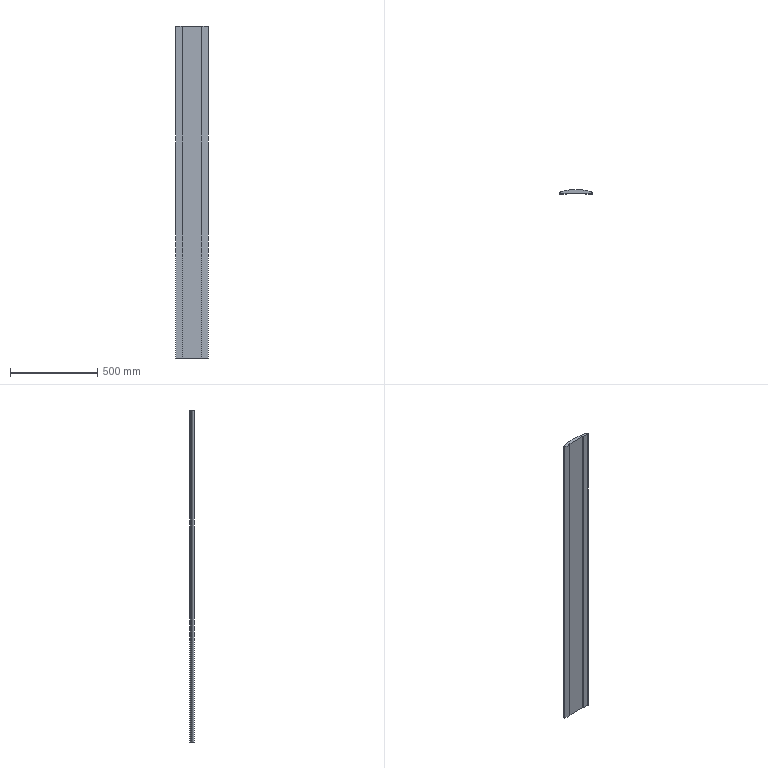Part | SolidWorks | features BaseBody 1 | 1 solid | 31 faces | box 188.037 x 25 x 1900 mm | volume 6268934 mm3 | cylinder 24 | plane 7 | commonest cylinder face diameters 0.2 x8 0.6 x6 661 x5 28 x3 0.4 x2
STEP:
#1=CARTESIAN_POINT('',(-94.018,0.7177,950.));
#2=VERTEX_POINT('',#1);
#3=CARTESIAN_POINT('',(-94.012,0.2909,950.));
#4=VERTEX_POINT('',#3);
#5=CARTESIAN_POINT('',(-80.018,0.7177,950.));
#6=DIRECTION('',(0.,0.,1.));
#7=DIRECTION('',(-1.,0.,0.));
#8=AXIS2_PLACEMENT_3D('',#5,#6,#7);
#9=CIRCLE('',#8,14.);
#10=EDGE_CURVE('',#2,#4,#9,.T.);
#11=ORIENTED_EDGE('',*,*,#10,.F.);
#12=CARTESIAN_POINT('',(-94.018,0.7177,-950.));
#13=VERTEX_POINT('',#12);
#14=CARTESIAN_POINT('',(-94.018,0.7177,950.));
#15=DIRECTION('',(0.,0.,-1.));
#16=VECTOR('',#15,1000.);
#17=LINE('',#14,#16);
#18=EDGE_CURVE('',#2,#13,#17,.T.);
#19=ORIENTED_EDGE('',*,*,#18,.T.);
#20=CARTESIAN_POINT('',(-94.012,0.2909,-950.));
#21=VERTEX_POINT('',#20);
#22=CARTESIAN_POINT('',(-80.018,0.7177,-950.));
#23=DIRECTION('',(0.,0.,1.));
#24=DIRECTION('',(-1.,0.,0.));
#25=AXIS2_PLACEMENT_3D('',#22,#23,#24);
#26=CIRCLE('',#25,14.);
#27=EDGE_CURVE('',#13,#21,#26,.T.);
#28=ORIENTED_EDGE('',*,*,#27,.T.);
#29=CARTESIAN_POINT('',(-94.012,0.2909,950.));
#30=DIRECTION('',(0.,0.,-1.));
#31=VECTOR('',#30,1000.);
#32=LINE('',#29,#31);
#33=EDGE_CURVE('',#4,#21,#32,.T.);
#34=ORIENTED_EDGE('',*,*,#33,.F.);
#35=EDGE_LOOP('',(#11,#19,#28,#34));
#36=FACE_OUTER_BOUND('',#35,.T.);
#37=CARTESIAN_POINT('',(-80.018,0.7177,950.));
#38=DIRECTION('',(0.,0.,-1.));
#39=DIRECTION('',(-1.,0.,0.));
#40=AXIS2_PLACEMENT_3D('',#37,#38,#39);
#41=CYLINDRICAL_SURFACE('',#40,14.);
#42=ADVANCED_FACE('',(#36),#41,.T.);
#43=CARTESIAN_POINT('',(-58.619,19.76,950.));
#44=VERTEX_POINT('',#43);
#45=CARTESIAN_POINT('',(58.619,19.76,950.));
#46=VERTEX_POINT('',#45);
#47=CARTESIAN_POINT('',(0.,-305.5,950.));
#48=DIRECTION('',(0.,0.,-1.));
#49=DIRECTION('',(-1.,0.,0.));
#50=AXIS2_PLACEMENT_3D('',#47,#48,#49);
#51=CIRCLE('',#50,330.5);
#52=EDGE_CURVE('',#44,#46,#51,.T.);
#53=ORIENTED_EDGE('',*,*,#52,.T.);
#54=CARTESIAN_POINT('',(58.619,19.76,-950.));
#55=VERTEX_POINT('',#54);
#56=CARTESIAN_POINT('',(58.619,19.76,950.));
#57=DIRECTION('',(0.,0.,-1.));
#58=VECTOR('',#57,1000.);
#59=LINE('',#56,#58);
#60=EDGE_CURVE('',#46,#55,#59,.T.);
#61=ORIENTED_EDGE('',*,*,#60,.T.);
#62=CARTESIAN_POINT('',(-58.619,19.76,-950.));
#63=VERTEX_POINT('',#62);
#64=CARTESIAN_POINT('',(0.,-305.5,-950.));
#65=DIRECTION('',(0.,0.,1.));
#66=DIRECTION('',(-1.,0.,0.));
#67=AXIS2_PLACEMENT_3D('',#64,#65,#66);
#68=CIRCLE('',#67,330.5);
#69=EDGE_CURVE('',#55,#63,#68,.T.);
#70=ORIENTED_EDGE('',*,*,#69,.T.);
#71=CARTESIAN_POINT('',(-58.619,19.76,950.));
#72=DIRECTION('',(0.,0.,1.));
#73=VECTOR('',#72,1000.);
#74=LINE('',#71,#73);
#75=EDGE_CURVE('',#63,#44,#74,.T.);
#76=ORIENTED_EDGE('',*,*,#75,.T.);
#77=EDGE_LOOP('',(#53,#61,#70,#76));
#78=FACE_OUTER_BOUND('',#77,.T.);
#79=CARTESIAN_POINT('',(0.,-305.5,950.));
#80=DIRECTION('',(0.,0.,-1.));
#81=DIRECTION('',(-1.,0.,0.));
#82=AXIS2_PLACEMENT_3D('',#79,#80,#81);
#83=CYLINDRICAL_SURFACE('',#82,330.5);
#84=ADVANCED_FACE('',(#78),#83,.T.);
#85=CARTESIAN_POINT('',(58.701,19.669,950.));
#86=VERTEX_POINT('',#85);
#87=CARTESIAN_POINT('',(58.601,19.662,950.));
#88=DIRECTION('',(0.,0.,-1.));
#89=DIRECTION('',(-1.,0.,0.));
#90=AXIS2_PLACEMENT_3D('',#87,#88,#89);
#91=CIRCLE('',#90,0.1);
#92=EDGE_CURVE('',#46,#86,#91,.T.);
#93=ORIENTED_EDGE('',*,*,#92,.T.);
#94=CARTESIAN_POINT('',(58.701,19.669,-950.));
#95=VERTEX_POINT('',#94);
#96=CARTESIAN_POINT('',(58.701,19.669,950.));
#97=DIRECTION('',(0.,0.,-1.));
#98=VECTOR('',#97,1000.);
#99=LINE('',#96,#98);
#100=EDGE_CURVE('',#86,#95,#99,.T.);
#101=ORIENTED_EDGE('',*,*,#100,.T.);
#102=CARTESIAN_POINT('',(58.601,19.662,-950.));
#103=DIRECTION('',(0.,0.,1.));
#104=DIRECTION('',(-1.,0.,0.));
#105=AXIS2_PLACEMENT_3D('',#102,#103,#104);
#106=CIRCLE('',#105,0.1);
#107=EDGE_CURVE('',#95,#55,#106,.T.);
#108=ORIENTED_EDGE('',*,*,#107,.T.);
#109=ORIENTED_EDGE('',*,*,#60,.F.);
#110=EDGE_LOOP('',(#93,#101,#108,#109));
#111=FACE_OUTER_BOUND('',#110,.T.);
#112=CARTESIAN_POINT('',(58.601,19.662,950.));
#113=DIRECTION('',(0.,0.,-1.));
#114=DIRECTION('',(-1.,0.,0.));
#115=AXIS2_PLACEMENT_3D('',#112,#113,#114);
#116=CYLINDRICAL_SURFACE('',#115,0.1);
#117=ADVANCED_FACE('',(#111),#116,.T.);
#118=CARTESIAN_POINT('',(-60.381,19.438,950.));
#119=VERTEX_POINT('',#118);
#120=CARTESIAN_POINT('',(-60.272,19.381,950.));
#121=VERTEX_POINT('',#120);
#122=CARTESIAN_POINT('',(-60.363,19.339,950.));
#123=DIRECTION('',(0.,0.,-1.));
#124=DIRECTION('',(-1.,0.,0.));
#125=AXIS2_PLACEMENT_3D('',#122,#123,#124);
#126=CIRCLE('',#125,0.1);
#127=EDGE_CURVE('',#119,#121,#126,.T.);
#128=ORIENTED_EDGE('',*,*,#127,.F.);
#129=CARTESIAN_POINT('',(-83.558,14.263,950.));
#130=VERTEX_POINT('',#129);
#131=CARTESIAN_POINT('',(0.,-305.5,950.));
#132=DIRECTION('',(0.,0.,1.));
#133=DIRECTION('',(-1.,0.,0.));
#134=AXIS2_PLACEMENT_3D('',#131,#132,#133);
#135=CIRCLE('',#134,330.5);
#136=EDGE_CURVE('',#119,#130,#135,.T.);
#137=ORIENTED_EDGE('',*,*,#136,.T.);
#138=CARTESIAN_POINT('',(-80.018,0.7177,950.));
#139=DIRECTION('',(0.,0.,1.));
#140=DIRECTION('',(-1.,0.,0.));
#141=AXIS2_PLACEMENT_3D('',#138,#139,#140);
#142=CIRCLE('',#141,14.);
#143=EDGE_CURVE('',#130,#2,#142,.T.);
#144=ORIENTED_EDGE('',*,*,#143,.T.);
#145=ORIENTED_EDGE('',*,*,#10,.T.);
#146=CARTESIAN_POINT('',(-93.712,0.,950.));
#147=VERTEX_POINT('',#146);
#148=CARTESIAN_POINT('',(-93.712,0.3,950.));
#149=DIRECTION('',(0.,0.,-1.));
#150=DIRECTION('',(-1.,0.,0.));
#151=AXIS2_PLACEMENT_3D('',#148,#149,#150);
#152=CIRCLE('',#151,0.3);
#153=EDGE_CURVE('',#147,#4,#152,.T.);
#154=ORIENTED_EDGE('',*,*,#153,.F.);
#155=CARTESIAN_POINT('',(-56.7,0.,950.));
#156=VERTEX_POINT('',#155);
#157=CARTESIAN_POINT('',(-80.018,0.,950.));
#158=DIRECTION('',(1.,0.,0.));
#159=VECTOR('',#158,1000.);
#160=LINE('',#157,#159);
#161=EDGE_CURVE('',#147,#156,#160,.T.);
#162=ORIENTED_EDGE('',*,*,#161,.T.);
#163=CARTESIAN_POINT('',(-56.5,0.2,950.));
#164=VERTEX_POINT('',#163);
#165=CARTESIAN_POINT('',(-56.7,0.2,950.));
#166=DIRECTION('',(0.,0.,-1.));
#167=DIRECTION('',(-1.,0.,0.));
#168=AXIS2_PLACEMENT_3D('',#165,#166,#167);
#169=CIRCLE('',#168,0.2);
#170=EDGE_CURVE('',#164,#156,#169,.T.);
#171=ORIENTED_EDGE('',*,*,#170,.F.);
#172=CARTESIAN_POINT('',(-56.5,4.5,950.));
#173=VERTEX_POINT('',#172);
#174=CARTESIAN_POINT('',(-56.5,0.7177,950.));
#175=DIRECTION('',(0.,1.,0.));
#176=VECTOR('',#175,1000.);
#177=LINE('',#174,#176);
#178=EDGE_CURVE('',#164,#173,#177,.T.);
#179=ORIENTED_EDGE('',*,*,#178,.T.);
#180=CARTESIAN_POINT('',(56.5,4.5,950.));
#181=VERTEX_POINT('',#180);
#182=CARTESIAN_POINT('',(-80.018,4.5,950.));
#183=DIRECTION('',(1.,0.,0.));
#184=VECTOR('',#183,1000.);
#185=LINE('',#182,#184);
#186=EDGE_CURVE('',#173,#181,#185,.T.);
#187=ORIENTED_EDGE('',*,*,#186,.T.);
#188=CARTESIAN_POINT('',(56.5,0.2,950.));
#189=VERTEX_POINT('',#188);
#190=CARTESIAN_POINT('',(56.5,0.7177,950.));
#191=DIRECTION('',(0.,-1.,0.));
#192=VECTOR('',#191,1000.);
#193=LINE('',#190,#192);
#194=EDGE_CURVE('',#181,#189,#193,.T.);
#195=ORIENTED_EDGE('',*,*,#194,.T.);
#196=CARTESIAN_POINT('',(56.7,0.,950.));
#197=VERTEX_POINT('',#196);
#198=CARTESIAN_POINT('',(56.7,0.2,950.));
#199=DIRECTION('',(0.,0.,-1.));
#200=DIRECTION('',(-1.,0.,0.));
#201=AXIS2_PLACEMENT_3D('',#198,#199,#200);
#202=CIRCLE('',#201,0.2);
#203=EDGE_CURVE('',#197,#189,#202,.T.);
#204=ORIENTED_EDGE('',*,*,#203,.F.);
#205=CARTESIAN_POINT('',(93.712,0.,950.));
#206=VERTEX_POINT('',#205);
#207=CARTESIAN_POINT('',(-80.018,0.,950.));
#208=DIRECTION('',(1.,0.,0.));
#209=VECTOR('',#208,1000.);
#210=LINE('',#207,#209);
#211=EDGE_CURVE('',#197,#206,#210,.T.);
#212=ORIENTED_EDGE('',*,*,#211,.T.);
#213=CARTESIAN_POINT('',(94.012,0.2909,950.));
#214=VERTEX_POINT('',#213);
#215=CARTESIAN_POINT('',(93.712,0.3,950.));
#216=DIRECTION('',(0.,0.,-1.));
#217=DIRECTION('',(-1.,0.,0.));
#218=AXIS2_PLACEMENT_3D('',#215,#216,#217);
#219=CIRCLE('',#218,0.3);
#220=EDGE_CURVE('',#214,#206,#219,.T.);
#221=ORIENTED_EDGE('',*,*,#220,.F.);
#222=CARTESIAN_POINT('',(83.558,14.263,950.));
#223=VERTEX_POINT('',#222);
#224=CARTESIAN_POINT('',(80.018,0.7177,950.));
#225=DIRECTION('',(0.,0.,1.));
#226=DIRECTION('',(-1.,0.,0.));
#227=AXIS2_PLACEMENT_3D('',#224,#225,#226);
#228=CIRCLE('',#227,14.);
#229=EDGE_CURVE('',#214,#223,#228,.T.);
#230=ORIENTED_EDGE('',*,*,#229,.T.);
#231=CARTESIAN_POINT('',(60.381,19.438,950.));
#232=VERTEX_POINT('',#231);
#233=CARTESIAN_POINT('',(0.,-305.5,950.));
#234=DIRECTION('',(0.,0.,1.));
#235=DIRECTION('',(-1.,0.,0.));
#236=AXIS2_PLACEMENT_3D('',#233,#234,#235);
#237=CIRCLE('',#236,330.5);
#238=EDGE_CURVE('',#223,#232,#237,.T.);
#239=ORIENTED_EDGE('',*,*,#238,.T.);
#240=CARTESIAN_POINT('',(60.272,19.381,950.));
#241=VERTEX_POINT('',#240);
#242=CARTESIAN_POINT('',(60.363,19.339,950.));
#243=DIRECTION('',(0.,0.,-1.));
#244=DIRECTION('',(-1.,0.,0.));
#245=AXIS2_PLACEMENT_3D('',#242,#243,#244);
#246=CIRCLE('',#245,0.1);
#247=EDGE_CURVE('',#241,#232,#246,.T.);
#248=ORIENTED_EDGE('',*,*,#247,.F.);
#249=CARTESIAN_POINT('',(59.701,19.487,950.));
#250=VERTEX_POINT('',#249);
#251=CARTESIAN_POINT('',(60.,19.508,950.));
#252=DIRECTION('',(0.,0.,-1.));
#253=DIRECTION('',(-1.,0.,0.));
#254=AXIS2_PLACEMENT_3D('',#251,#252,#253);
#255=CIRCLE('',#254,0.3);
#256=EDGE_CURVE('',#241,#250,#255,.T.);
#257=ORIENTED_EDGE('',*,*,#256,.T.);
#258=CARTESIAN_POINT('',(59.619,19.578,950.));
#259=VERTEX_POINT('',#258);
#260=CARTESIAN_POINT('',(59.601,19.48,950.));
#261=DIRECTION('',(0.,0.,-1.));
#262=DIRECTION('',(-1.,0.,0.));
#263=AXIS2_PLACEMENT_3D('',#260,#261,#262);
#264=CIRCLE('',#263,0.1);
#265=EDGE_CURVE('',#259,#250,#264,.T.);
#266=ORIENTED_EDGE('',*,*,#265,.F.);
#267=CARTESIAN_POINT('',(59.381,19.622,950.));
#268=VERTEX_POINT('',#267);
#269=CARTESIAN_POINT('',(0.,-305.5,950.));
#270=DIRECTION('',(0.,0.,-1.));
#271=DIRECTION('',(-1.,0.,0.));
#272=AXIS2_PLACEMENT_3D('',#269,#270,#271);
#273=CIRCLE('',#272,330.5);
#274=EDGE_CURVE('',#268,#259,#273,.T.);
#275=ORIENTED_EDGE('',*,*,#274,.F.);
#276=CARTESIAN_POINT('',(59.272,19.565,950.));
#277=VERTEX_POINT('',#276);
#278=CARTESIAN_POINT('',(59.363,19.523,950.));
#279=DIRECTION('',(0.,0.,-1.));
#280=DIRECTION('',(-1.,0.,0.));
#281=AXIS2_PLACEMENT_3D('',#278,#279,#280);
#282=CIRCLE('',#281,0.1);
#283=EDGE_CURVE('',#277,#268,#282,.T.);
#284=ORIENTED_EDGE('',*,*,#283,.F.);
#285=CARTESIAN_POINT('',(59.,19.691,950.));
#286=DIRECTION('',(0.,0.,-1.));
#287=DIRECTION('',(-1.,0.,0.));
#288=AXIS2_PLACEMENT_3D('',#285,#286,#287);
#289=CIRCLE('',#288,0.3);
#290=EDGE_CURVE('',#277,#86,#289,.T.);
#291=ORIENTED_EDGE('',*,*,#290,.T.);
#292=ORIENTED_EDGE('',*,*,#92,.F.);
#293=ORIENTED_EDGE('',*,*,#52,.F.);
#294=CARTESIAN_POINT('',(-58.701,19.669,950.));
#295=VERTEX_POINT('',#294);
#296=CARTESIAN_POINT('',(-58.601,19.662,950.));
#297=DIRECTION('',(0.,0.,1.));
#298=DIRECTION('',(-1.,0.,0.));
#299=AXIS2_PLACEMENT_3D('',#296,#297,#298);
#300=CIRCLE('',#299,0.1);
#301=EDGE_CURVE('',#44,#295,#300,.T.);
#302=ORIENTED_EDGE('',*,*,#301,.T.);
#303=CARTESIAN_POINT('',(-59.272,19.565,950.));
#304=VERTEX_POINT('',#303);
#305=CARTESIAN_POINT('',(-59.,19.691,950.));
#306=DIRECTION('',(0.,0.,-1.));
#307=DIRECTION('',(-1.,0.,0.));
#308=AXIS2_PLACEMENT_3D('',#305,#306,#307);
#309=CIRCLE('',#308,0.3);
#310=EDGE_CURVE('',#295,#304,#309,.T.);
#311=ORIENTED_EDGE('',*,*,#310,.T.);
#312=CARTESIAN_POINT('',(-59.381,19.622,950.));
#313=VERTEX_POINT('',#312);
#314=CARTESIAN_POINT('',(-59.363,19.523,950.));
#315=DIRECTION('',(0.,0.,-1.));
#316=DIRECTION('',(-1.,0.,0.));
#317=AXIS2_PLACEMENT_3D('',#314,#315,#316);
#318=CIRCLE('',#317,0.1);
#319=EDGE_CURVE('',#313,#304,#318,.T.);
#320=ORIENTED_EDGE('',*,*,#319,.F.);
#321=CARTESIAN_POINT('',(-59.619,19.578,950.));
#322=VERTEX_POINT('',#321);
#323=CARTESIAN_POINT('',(0.,-305.5,950.));
#324=DIRECTION('',(0.,0.,-1.));
#325=DIRECTION('',(-1.,0.,0.));
#326=AXIS2_PLACEMENT_3D('',#323,#324,#325);
#327=CIRCLE('',#326,330.5);
#328=EDGE_CURVE('',#322,#313,#327,.T.);
#329=ORIENTED_EDGE('',*,*,#328,.F.);
#330=CARTESIAN_POINT('',(-59.701,19.487,950.));
#331=VERTEX_POINT('',#330);
#332=CARTESIAN_POINT('',(-59.601,19.48,950.));
#333=DIRECTION('',(0.,0.,-1.));
#334=DIRECTION('',(-1.,0.,0.));
#335=AXIS2_PLACEMENT_3D('',#332,#333,#334);
#336=CIRCLE('',#335,0.1);
#337=EDGE_CURVE('',#331,#322,#336,.T.);
#338=ORIENTED_EDGE('',*,*,#337,.F.);
#339=CARTESIAN_POINT('',(-60.,19.508,950.));
#340=DIRECTION('',(0.,0.,-1.));
#341=DIRECTION('',(-1.,0.,0.));
#342=AXIS2_PLACEMENT_3D('',#339,#340,#341);
#343=CIRCLE('',#342,0.3);
#344=EDGE_CURVE('',#331,#121,#343,.T.);
#345=ORIENTED_EDGE('',*,*,#344,.T.);
#346=EDGE_LOOP('',(#128,#137,#144,#145,#154,#162,#171,#179,#187,#195,#204,#212,#221,#230,#239,#248,#257,#266,#275,#284,#291,#292,#293,#302,#311,#320,#329,#338,#345));
#347=FACE_OUTER_BOUND('',#346,.T.);
#348=CARTESIAN_POINT('',(-80.018,0.7177,950.));
#349=DIRECTION('',(0.,0.,1.));
#350=DIRECTION('',(1.,0.,0.));
#351=AXIS2_PLACEMENT_3D('',#348,#349,#350);
#352=PLANE('',#351);
#353=ADVANCED_FACE('',(#347),#352,.T.);
#354=ORIENTED_EDGE('',*,*,#301,.F.);
#355=ORIENTED_EDGE('',*,*,#75,.F.);
#356=CARTESIAN_POINT('',(-58.701,19.669,-950.));
#357=VERTEX_POINT('',#356);
#358=CARTESIAN_POINT('',(-58.601,19.662,-950.));
#359=DIRECTION('',(0.,0.,1.));
#360=DIRECTION('',(-1.,0.,0.));
#361=AXIS2_PLACEMENT_3D('',#358,#359,#360);
#362=CIRCLE('',#361,0.1);
#363=EDGE_CURVE('',#63,#357,#362,.T.);
#364=ORIENTED_EDGE('',*,*,#363,.T.);
#365=CARTESIAN_POINT('',(-58.701,19.669,950.));
#366=DIRECTION('',(0.,0.,1.));
#367=VECTOR('',#366,1000.);
#368=LINE('',#365,#367);
#369=EDGE_CURVE('',#357,#295,#368,.T.);
#370=ORIENTED_EDGE('',*,*,#369,.T.);
#371=EDGE_LOOP('',(#354,#355,#364,#370));
#372=FACE_OUTER_BOUND('',#371,.T.);
#373=CARTESIAN_POINT('',(-58.601,19.662,950.));
#374=DIRECTION('',(0.,0.,-1.));
#375=DIRECTION('',(-1.,0.,0.));
#376=AXIS2_PLACEMENT_3D('',#373,#374,#375);
#377=CYLINDRICAL_SURFACE('',#376,0.1);
#378=ADVANCED_FACE('',(#372),#377,.T.);
#379=CARTESIAN_POINT('',(-93.712,0.,-950.));
#380=VERTEX_POINT('',#379);
#381=CARTESIAN_POINT('',(-93.712,0.3,-950.));
#382=DIRECTION('',(0.,0.,1.));
#383=DIRECTION('',(-1.,0.,0.));
#384=AXIS2_PLACEMENT_3D('',#381,#382,#383);
#385=CIRCLE('',#384,0.3);
#386=EDGE_CURVE('',#21,#380,#385,.T.);
#387=ORIENTED_EDGE('',*,*,#386,.F.);
#388=ORIENTED_EDGE('',*,*,#27,.F.);
#389=CARTESIAN_POINT('',(-83.558,14.263,-950.));
#390=VERTEX_POINT('',#389);
#391=CARTESIAN_POINT('',(-80.018,0.7177,-950.));
#392=DIRECTION('',(0.,0.,1.));
#393=DIRECTION('',(-1.,0.,0.));
#394=AXIS2_PLACEMENT_3D('',#391,#392,#393);
#395=CIRCLE('',#394,14.);
#396=EDGE_CURVE('',#390,#13,#395,.T.);
#397=ORIENTED_EDGE('',*,*,#396,.F.);
#398=CARTESIAN_POINT('',(-60.381,19.438,-950.));
#399=VERTEX_POINT('',#398);
#400=CARTESIAN_POINT('',(0.,-305.5,-950.));
#401=DIRECTION('',(0.,0.,1.));
#402=DIRECTION('',(-1.,0.,0.));
#403=AXIS2_PLACEMENT_3D('',#400,#401,#402);
#404=CIRCLE('',#403,330.5);
#405=EDGE_CURVE('',#399,#390,#404,.T.);
#406=ORIENTED_EDGE('',*,*,#405,.F.);
#407=CARTESIAN_POINT('',(-60.272,19.381,-950.));
#408=VERTEX_POINT('',#407);
#409=CARTESIAN_POINT('',(-60.363,19.339,-950.));
#410=DIRECTION('',(0.,0.,1.));
#411=DIRECTION('',(-1.,0.,0.));
#412=AXIS2_PLACEMENT_3D('',#409,#410,#411);
#413=CIRCLE('',#412,0.1);
#414=EDGE_CURVE('',#408,#399,#413,.T.);
#415=ORIENTED_EDGE('',*,*,#414,.F.);
#416=CARTESIAN_POINT('',(-59.701,19.487,-950.));
#417=VERTEX_POINT('',#416);
#418=CARTESIAN_POINT('',(-60.,19.508,-950.));
#419=DIRECTION('',(0.,0.,1.));
#420=DIRECTION('',(-1.,0.,0.));
#421=AXIS2_PLACEMENT_3D('',#418,#419,#420);
#422=CIRCLE('',#421,0.3);
#423=EDGE_CURVE('',#408,#417,#422,.T.);
#424=ORIENTED_EDGE('',*,*,#423,.T.);
#425=CARTESIAN_POINT('',(-59.619,19.578,-950.));
#426=VERTEX_POINT('',#425);
#427=CARTESIAN_POINT('',(-59.601,19.48,-950.));
#428=DIRECTION('',(0.,0.,1.));
#429=DIRECTION('',(-1.,0.,0.));
#430=AXIS2_PLACEMENT_3D('',#427,#428,#429);
#431=CIRCLE('',#430,0.1);
#432=EDGE_CURVE('',#426,#417,#431,.T.);
#433=ORIENTED_EDGE('',*,*,#432,.F.);
#434=CARTESIAN_POINT('',(-59.381,19.622,-950.));
#435=VERTEX_POINT('',#434);
#436=CARTESIAN_POINT('',(0.,-305.5,-950.));
#437=DIRECTION('',(0.,0.,1.));
#438=DIRECTION('',(-1.,0.,0.));
#439=AXIS2_PLACEMENT_3D('',#436,#437,#438);
#440=CIRCLE('',#439,330.5);
#441=EDGE_CURVE('',#435,#426,#440,.T.);
#442=ORIENTED_EDGE('',*,*,#441,.F.);
#443=CARTESIAN_POINT('',(-59.272,19.565,-950.));
#444=VERTEX_POINT('',#443);
#445=CARTESIAN_POINT('',(-59.363,19.523,-950.));
#446=DIRECTION('',(0.,0.,1.));
#447=DIRECTION('',(-1.,0.,0.));
#448=AXIS2_PLACEMENT_3D('',#445,#446,#447);
#449=CIRCLE('',#448,0.1);
#450=EDGE_CURVE('',#444,#435,#449,.T.);
#451=ORIENTED_EDGE('',*,*,#450,.F.);
#452=CARTESIAN_POINT('',(-59.,19.691,-950.));
#453=DIRECTION('',(0.,0.,-1.));
#454=DIRECTION('',(-1.,0.,0.));
#455=AXIS2_PLACEMENT_3D('',#452,#453,#454);
#456=CIRCLE('',#455,0.3);
#457=EDGE_CURVE('',#357,#444,#456,.T.);
#458=ORIENTED_EDGE('',*,*,#457,.F.);
#459=ORIENTED_EDGE('',*,*,#363,.F.);
#460=ORIENTED_EDGE('',*,*,#69,.F.);
#461=ORIENTED_EDGE('',*,*,#107,.F.);
#462=CARTESIAN_POINT('',(59.272,19.565,-950.));
#463=VERTEX_POINT('',#462);
#464=CARTESIAN_POINT('',(59.,19.691,-950.));
#465=DIRECTION('',(0.,0.,-1.));
#466=DIRECTION('',(-1.,0.,0.));
#467=AXIS2_PLACEMENT_3D('',#464,#465,#466);
#468=CIRCLE('',#467,0.3);
#469=EDGE_CURVE('',#463,#95,#468,.T.);
#470=ORIENTED_EDGE('',*,*,#469,.F.);
#471=CARTESIAN_POINT('',(59.381,19.622,-950.));
#472=VERTEX_POINT('',#471);
#473=CARTESIAN_POINT('',(59.363,19.523,-950.));
#474=DIRECTION('',(0.,0.,1.));
#475=DIRECTION('',(-1.,0.,0.));
#476=AXIS2_PLACEMENT_3D('',#473,#474,#475);
#477=CIRCLE('',#476,0.1);
#478=EDGE_CURVE('',#472,#463,#477,.T.);
#479=ORIENTED_EDGE('',*,*,#478,.F.);
#480=CARTESIAN_POINT('',(59.619,19.578,-950.));
#481=VERTEX_POINT('',#480);
#482=CARTESIAN_POINT('',(0.,-305.5,-950.));
#483=DIRECTION('',(0.,0.,1.));
#484=DIRECTION('',(-1.,0.,0.));
#485=AXIS2_PLACEMENT_3D('',#482,#483,#484);
#486=CIRCLE('',#485,330.5);
#487=EDGE_CURVE('',#481,#472,#486,.T.);
#488=ORIENTED_EDGE('',*,*,#487,.F.);
#489=CARTESIAN_POINT('',(59.701,19.487,-950.));
#490=VERTEX_POINT('',#489);
#491=CARTESIAN_POINT('',(59.601,19.48,-950.));
#492=DIRECTION('',(0.,0.,1.));
#493=DIRECTION('',(-1.,0.,0.));
#494=AXIS2_PLACEMENT_3D('',#491,#492,#493);
#495=CIRCLE('',#494,0.1);
#496=EDGE_CURVE('',#490,#481,#495,.T.);
#497=ORIENTED_EDGE('',*,*,#496,.F.);
#498=CARTESIAN_POINT('',(60.272,19.381,-950.));
#499=VERTEX_POINT('',#498);
#500=CARTESIAN_POINT('',(60.,19.508,-950.));
#501=DIRECTION('',(0.,0.,1.));
#502=DIRECTION('',(-1.,0.,0.));
#503=AXIS2_PLACEMENT_3D('',#500,#501,#502);
#504=CIRCLE('',#503,0.3);
#505=EDGE_CURVE('',#490,#499,#504,.T.);
#506=ORIENTED_EDGE('',*,*,#505,.T.);
#507=CARTESIAN_POINT('',(60.381,19.438,-950.));
#508=VERTEX_POINT('',#507);
#509=CARTESIAN_POINT('',(60.363,19.339,-950.));
#510=DIRECTION('',(0.,0.,1.));
#511=DIRECTION('',(-1.,0.,0.));
#512=AXIS2_PLACEMENT_3D('',#509,#510,#511);
#513=CIRCLE('',#512,0.1);
#514=EDGE_CURVE('',#508,#499,#513,.T.);
#515=ORIENTED_EDGE('',*,*,#514,.F.);
#516=CARTESIAN_POINT('',(83.558,14.263,-950.));
#517=VERTEX_POINT('',#516);
#518=CARTESIAN_POINT('',(0.,-305.5,-950.));
#519=DIRECTION('',(0.,0.,1.));
#520=DIRECTION('',(-1.,0.,0.));
#521=AXIS2_PLACEMENT_3D('',#518,#519,#520);
#522=CIRCLE('',#521,330.5);
#523=EDGE_CURVE('',#517,#508,#522,.T.);
#524=ORIENTED_EDGE('',*,*,#523,.F.);
#525=CARTESIAN_POINT('',(94.012,0.2909,-950.));
#526=VERTEX_POINT('',#525);
#527=CARTESIAN_POINT('',(80.018,0.7177,-950.));
#528=DIRECTION('',(0.,0.,1.));
#529=DIRECTION('',(-1.,0.,0.));
#530=AXIS2_PLACEMENT_3D('',#527,#528,#529);
#531=CIRCLE('',#530,14.);
#532=EDGE_CURVE('',#526,#517,#531,.T.);
#533=ORIENTED_EDGE('',*,*,#532,.F.);
#534=CARTESIAN_POINT('',(93.712,0.,-950.));
#535=VERTEX_POINT('',#534);
#536=CARTESIAN_POINT('',(93.712,0.3,-950.));
#537=DIRECTION('',(0.,0.,1.));
#538=DIRECTION('',(-1.,0.,0.));
#539=AXIS2_PLACEMENT_3D('',#536,#537,#538);
#540=CIRCLE('',#539,0.3);
#541=EDGE_CURVE('',#535,#526,#540,.T.);
#542=ORIENTED_EDGE('',*,*,#541,.F.);
#543=CARTESIAN_POINT('',(56.7,0.,-950.));
#544=VERTEX_POINT('',#543);
#545=CARTESIAN_POINT('',(-80.018,0.,-950.));
#546=DIRECTION('',(1.,0.,0.));
#547=VECTOR('',#546,1000.);
#548=LINE('',#545,#547);
#549=EDGE_CURVE('',#544,#535,#548,.T.);
#550=ORIENTED_EDGE('',*,*,#549,.F.);
#551=CARTESIAN_POINT('',(56.5,0.2,-950.));
#552=VERTEX_POINT('',#551);
#553=CARTESIAN_POINT('',(56.7,0.2,-950.));
#554=DIRECTION('',(0.,0.,1.));
#555=DIRECTION('',(-1.,0.,0.));
#556=AXIS2_PLACEMENT_3D('',#553,#554,#555);
#557=CIRCLE('',#556,0.2);
#558=EDGE_CURVE('',#552,#544,#557,.T.);
#559=ORIENTED_EDGE('',*,*,#558,.F.);
#560=CARTESIAN_POINT('',(56.5,4.5,-950.));
#561=VERTEX_POINT('',#560);
#562=CARTESIAN_POINT('',(56.5,0.7177,-950.));
#563=DIRECTION('',(0.,-1.,0.));
#564=VECTOR('',#563,1000.);
#565=LINE('',#562,#564);
#566=EDGE_CURVE('',#561,#552,#565,.T.);
#567=ORIENTED_EDGE('',*,*,#566,.F.);
#568=CARTESIAN_POINT('',(-56.5,4.5,-950.));
#569=VERTEX_POINT('',#568);
#570=CARTESIAN_POINT('',(-80.018,4.5,-950.));
#571=DIRECTION('',(1.,0.,0.));
#572=VECTOR('',#571,1000.);
#573=LINE('',#570,#572);
#574=EDGE_CURVE('',#569,#561,#573,.T.);
#575=ORIENTED_EDGE('',*,*,#574,.F.);
#576=CARTESIAN_POINT('',(-56.5,0.2,-950.));
#577=VERTEX_POINT('',#576);
#578=CARTESIAN_POINT('',(-56.5,0.7177,-950.));
#579=DIRECTION('',(0.,1.,0.));
#580=VECTOR('',#579,1000.);
#581=LINE('',#578,#580);
#582=EDGE_CURVE('',#577,#569,#581,.T.);
#583=ORIENTED_EDGE('',*,*,#582,.F.);
#584=CARTESIAN_POINT('',(-56.7,0.,-950.));
#585=VERTEX_POINT('',#584);
#586=CARTESIAN_POINT('',(-56.7,0.2,-950.));
#587=DIRECTION('',(0.,0.,1.));
#588=DIRECTION('',(-1.,0.,0.));
#589=AXIS2_PLACEMENT_3D('',#586,#587,#588);
#590=CIRCLE('',#589,0.2);
#591=EDGE_CURVE('',#585,#577,#590,.T.);
#592=ORIENTED_EDGE('',*,*,#591,.F.);
#593=CARTESIAN_POINT('',(-80.018,0.,-950.));
#594=DIRECTION('',(1.,0.,0.));
#595=VECTOR('',#594,1000.);
#596=LINE('',#593,#595);
#597=EDGE_CURVE('',#380,#585,#596,.T.);
#598=ORIENTED_EDGE('',*,*,#597,.F.);
#599=EDGE_LOOP('',(#387,#388,#397,#406,#415,#424,#433,#442,#451,#458,#459,#460,#461,#470,#479,#488,#497,#506,#515,#524,#533,#542,#550,#559,#567,#575,#583,#592,#598));
#600=FACE_OUTER_BOUND('',#599,.T.);
#601=CARTESIAN_POINT('',(-80.018,0.7177,-950.));
#602=DIRECTION('',(0.,0.,1.));
#603=DIRECTION('',(1.,0.,0.));
#604=AXIS2_PLACEMENT_3D('',#601,#602,#603);
#605=PLANE('',#604);
#606=ADVANCED_FACE('',(#600),#605,.F.);
#607=ORIENTED_EDGE('',*,*,#100,.F.);
#608=ORIENTED_EDGE('',*,*,#290,.F.);
#609=CARTESIAN_POINT('',(59.272,19.565,950.));
#610=DIRECTION('',(0.,0.,1.));
#611=VECTOR('',#610,1000.);
#612=LINE('',#609,#611);
#613=EDGE_CURVE('',#463,#277,#612,.T.);
#614=ORIENTED_EDGE('',*,*,#613,.F.);
#615=ORIENTED_EDGE('',*,*,#469,.T.);
#616=EDGE_LOOP('',(#607,#608,#614,#615));
#617=FACE_OUTER_BOUND('',#616,.T.);
#618=CARTESIAN_POINT('',(59.,19.691,950.));
#619=DIRECTION('',(0.,0.,-1.));
#620=DIRECTION('',(-1.,0.,0.));
#621=AXIS2_PLACEMENT_3D('',#618,#619,#620);
#622=CYLINDRICAL_SURFACE('',#621,0.3);
#623=ADVANCED_FACE('',(#617),#622,.F.);
#624=ORIENTED_EDGE('',*,*,#136,.F.);
#625=CARTESIAN_POINT('',(-60.381,19.438,950.));
#626=DIRECTION('',(0.,0.,-1.));
#627=VECTOR('',#626,1000.);
#628=LINE('',#625,#627);
#629=EDGE_CURVE('',#119,#399,#628,.T.);
#630=ORIENTED_EDGE('',*,*,#629,.T.);
#631=ORIENTED_EDGE('',*,*,#405,.T.);
#632=CARTESIAN_POINT('',(-83.558,14.263,950.));
#633=DIRECTION('',(0.,0.,1.));
#634=VECTOR('',#633,1000.);
#635=LINE('',#632,#634);
#636=EDGE_CURVE('',#390,#130,#635,.T.);
#637=ORIENTED_EDGE('',*,*,#636,.T.);
#638=EDGE_LOOP('',(#624,#630,#631,#637));
#639=FACE_OUTER_BOUND('',#638,.T.);
#640=CARTESIAN_POINT('',(0.,-305.5,950.));
#641=DIRECTION('',(0.,0.,-1.));
#642=DIRECTION('',(-1.,0.,0.));
#643=AXIS2_PLACEMENT_3D('',#640,#641,#642);
#644=CYLINDRICAL_SURFACE('',#643,330.5);
#645=ADVANCED_FACE('',(#639),#644,.T.);
#646=ORIENTED_EDGE('',*,*,#238,.F.);
#647=CARTESIAN_POINT('',(83.558,14.263,950.));
#648=DIRECTION('',(0.,0.,-1.));
#649=VECTOR('',#648,1000.);
#650=LINE('',#647,#649);
#651=EDGE_CURVE('',#223,#517,#650,.T.);
#652=ORIENTED_EDGE('',*,*,#651,.T.);
#653=ORIENTED_EDGE('',*,*,#523,.T.);
#654=CARTESIAN_POINT('',(60.381,19.438,950.));
#655=DIRECTION('',(0.,0.,1.));
#656=VECTOR('',#655,1000.);
#657=LINE('',#654,#656);
#658=EDGE_CURVE('',#508,#232,#657,.T.);
#659=ORIENTED_EDGE('',*,*,#658,.T.);
#660=EDGE_LOOP('',(#646,#652,#653,#659));
#661=FACE_OUTER_BOUND('',#660,.T.);
#662=CARTESIAN_POINT('',(0.,-305.5,950.));
#663=DIRECTION('',(0.,0.,-1.));
#664=DIRECTION('',(-1.,0.,0.));
#665=AXIS2_PLACEMENT_3D('',#662,#663,#664);
#666=CYLINDRICAL_SURFACE('',#665,330.5);
#667=ADVANCED_FACE('',(#661),#666,.T.);
#668=ORIENTED_EDGE('',*,*,#532,.T.);
#669=ORIENTED_EDGE('',*,*,#651,.F.);
#670=ORIENTED_EDGE('',*,*,#229,.F.);
#671=CARTESIAN_POINT('',(94.012,0.2909,950.));
#672=DIRECTION('',(0.,0.,-1.));
#673=VECTOR('',#672,1000.);
#674=LINE('',#671,#673);
#675=EDGE_CURVE('',#214,#526,#674,.T.);
#676=ORIENTED_EDGE('',*,*,#675,.T.);
#677=EDGE_LOOP('',(#668,#669,#670,#676));
#678=FACE_OUTER_BOUND('',#677,.T.);
#679=CARTESIAN_POINT('',(80.018,0.7177,950.));
#680=DIRECTION('',(0.,0.,-1.));
#681=DIRECTION('',(-1.,0.,0.));
#682=AXIS2_PLACEMENT_3D('',#679,#680,#681);
#683=CYLINDRICAL_SURFACE('',#682,14.);
#684=ADVANCED_FACE('',(#678),#683,.T.);
#685=CARTESIAN_POINT('',(93.712,0.,950.));
#686=DIRECTION('',(0.,0.,-1.));
#687=VECTOR('',#686,1000.);
#688=LINE('',#685,#687);
#689=EDGE_CURVE('',#206,#535,#688,.T.);
#690=ORIENTED_EDGE('',*,*,#689,.F.);
#691=ORIENTED_EDGE('',*,*,#211,.F.);
#692=CARTESIAN_POINT('',(56.7,0.,950.));
#693=DIRECTION('',(0.,0.,1.));
#694=VECTOR('',#693,1000.);
#695=LINE('',#692,#694);
#696=EDGE_CURVE('',#544,#197,#695,.T.);
#697=ORIENTED_EDGE('',*,*,#696,.F.);
#698=ORIENTED_EDGE('',*,*,#549,.T.);
#699=EDGE_LOOP('',(#690,#691,#697,#698));
#700=FACE_OUTER_BOUND('',#699,.T.);
#701=CARTESIAN_POINT('',(94.,0.,950.));
#702=DIRECTION('',(0.,1.,0.));
#703=DIRECTION('',(-1.,0.,0.));
#704=AXIS2_PLACEMENT_3D('',#701,#702,#703);
#705=PLANE('',#704);
#706=ADVANCED_FACE('',(#700),#705,.F.);
#707=CARTESIAN_POINT('',(56.5,0.2,950.));
#708=DIRECTION('',(0.,0.,-1.));
#709=VECTOR('',#708,1000.);
#710=LINE('',#707,#709);
#711=EDGE_CURVE('',#189,#552,#710,.T.);
#712=ORIENTED_EDGE('',*,*,#711,.F.);
#713=ORIENTED_EDGE('',*,*,#194,.F.);
#714=CARTESIAN_POINT('',(56.5,4.5,950.));
#715=DIRECTION('',(0.,0.,1.));
#716=VECTOR('',#715,1000.);
#717=LINE('',#714,#716);
#718=EDGE_CURVE('',#561,#181,#717,.T.);
#719=ORIENTED_EDGE('',*,*,#718,.F.);
#720=ORIENTED_EDGE('',*,*,#566,.T.);
#721=EDGE_LOOP('',(#712,#713,#719,#720));
#722=FACE_OUTER_BOUND('',#721,.T.);
#723=CARTESIAN_POINT('',(56.5,0.2,950.));
#724=DIRECTION('',(1.,0.,0.));
#725=DIRECTION('',(0.,1.,0.));
#726=AXIS2_PLACEMENT_3D('',#723,#724,#725);
#727=PLANE('',#726);
#728=ADVANCED_FACE('',(#722),#727,.F.);
#729=ORIENTED_EDGE('',*,*,#718,.T.);
#730=ORIENTED_EDGE('',*,*,#186,.F.);
#731=CARTESIAN_POINT('',(-56.5,4.5,950.));
#732=DIRECTION('',(0.,0.,1.));
#733=VECTOR('',#732,1000.);
#734=LINE('',#731,#733);
#735=EDGE_CURVE('',#569,#173,#734,.T.);
#736=ORIENTED_EDGE('',*,*,#735,.F.);
#737=ORIENTED_EDGE('',*,*,#574,.T.);
#738=EDGE_LOOP('',(#729,#730,#736,#737));
#739=FACE_OUTER_BOUND('',#738,.T.);
#740=CARTESIAN_POINT('',(-56.5,4.5,950.));
#741=DIRECTION('',(0.,1.,0.));
#742=DIRECTION('',(-1.,0.,0.));
#743=AXIS2_PLACEMENT_3D('',#740,#741,#742);
#744=PLANE('',#743);
#745=ADVANCED_FACE('',(#739),#744,.F.);
#746=ORIENTED_EDGE('',*,*,#735,.T.);
#747=ORIENTED_EDGE('',*,*,#178,.F.);
#748=CARTESIAN_POINT('',(-56.5,0.2,950.));
#749=DIRECTION('',(0.,0.,1.));
#750=VECTOR('',#749,1000.);
#751=LINE('',#748,#750);
#752=EDGE_CURVE('',#577,#164,#751,.T.);
#753=ORIENTED_EDGE('',*,*,#752,.F.);
#754=ORIENTED_EDGE('',*,*,#582,.T.);
#755=EDGE_LOOP('',(#746,#747,#753,#754));
#756=FACE_OUTER_BOUND('',#755,.T.);
#757=CARTESIAN_POINT('',(-56.5,0.2,950.));
#758=DIRECTION('',(-1.,0.,0.));
#759=DIRECTION('',(0.,-1.,0.));
#760=AXIS2_PLACEMENT_3D('',#757,#758,#759);
#761=PLANE('',#760);
#762=ADVANCED_FACE('',(#756),#761,.F.);
#763=CARTESIAN_POINT('',(-93.712,0.,950.));
#764=DIRECTION('',(0.,0.,1.));
#765=VECTOR('',#764,1000.);
#766=LINE('',#763,#765);
#767=EDGE_CURVE('',#380,#147,#766,.T.);
#768=ORIENTED_EDGE('',*,*,#767,.F.);
#769=ORIENTED_EDGE('',*,*,#597,.T.);
#770=CARTESIAN_POINT('',(-56.7,0.,950.));
#771=DIRECTION('',(0.,0.,-1.));
#772=VECTOR('',#771,1000.);
#773=LINE('',#770,#772);
#774=EDGE_CURVE('',#156,#585,#773,.T.);
#775=ORIENTED_EDGE('',*,*,#774,.F.);
#776=ORIENTED_EDGE('',*,*,#161,.F.);
#777=EDGE_LOOP('',(#768,#769,#775,#776));
#778=FACE_OUTER_BOUND('',#777,.T.);
#779=CARTESIAN_POINT('',(-56.7,0.,950.));
#780=DIRECTION('',(0.,1.,0.));
#781=DIRECTION('',(-1.,0.,0.));
#782=AXIS2_PLACEMENT_3D('',#779,#780,#781);
#783=PLANE('',#782);
#784=ADVANCED_FACE('',(#778),#783,.F.);
#785=ORIENTED_EDGE('',*,*,#18,.F.);
#786=ORIENTED_EDGE('',*,*,#143,.F.);
#787=ORIENTED_EDGE('',*,*,#636,.F.);
#788=ORIENTED_EDGE('',*,*,#396,.T.);
#789=EDGE_LOOP('',(#785,#786,#787,#788));
#790=FACE_OUTER_BOUND('',#789,.T.);
#791=CARTESIAN_POINT('',(-80.018,0.7177,950.));
#792=DIRECTION('',(0.,0.,-1.));
#793=DIRECTION('',(-1.,0.,0.));
#794=AXIS2_PLACEMENT_3D('',#791,#792,#793);
#795=CYLINDRICAL_SURFACE('',#794,14.);
#796=ADVANCED_FACE('',(#790),#795,.T.);
#797=CARTESIAN_POINT('',(-59.272,19.565,950.));
#798=DIRECTION('',(0.,0.,-1.));
#799=VECTOR('',#798,1000.);
#800=LINE('',#797,#799);
#801=EDGE_CURVE('',#304,#444,#800,.T.);
#802=ORIENTED_EDGE('',*,*,#801,.F.);
#803=ORIENTED_EDGE('',*,*,#310,.F.);
#804=ORIENTED_EDGE('',*,*,#369,.F.);
#805=ORIENTED_EDGE('',*,*,#457,.T.);
#806=EDGE_LOOP('',(#802,#803,#804,#805));
#807=FACE_OUTER_BOUND('',#806,.T.);
#808=CARTESIAN_POINT('',(-59.,19.691,950.));
#809=DIRECTION('',(0.,0.,-1.));
#810=DIRECTION('',(-1.,0.,0.));
#811=AXIS2_PLACEMENT_3D('',#808,#809,#810);
#812=CYLINDRICAL_SURFACE('',#811,0.3);
#813=ADVANCED_FACE('',(#807),#812,.F.);
#814=ORIENTED_EDGE('',*,*,#283,.T.);
#815=CARTESIAN_POINT('',(59.381,19.622,950.));
#816=DIRECTION('',(0.,0.,-1.));
#817=VECTOR('',#816,1000.);
#818=LINE('',#815,#817);
#819=EDGE_CURVE('',#268,#472,#818,.T.);
#820=ORIENTED_EDGE('',*,*,#819,.T.);
#821=ORIENTED_EDGE('',*,*,#478,.T.);
#822=ORIENTED_EDGE('',*,*,#613,.T.);
#823=EDGE_LOOP('',(#814,#820,#821,#822));
#824=FACE_OUTER_BOUND('',#823,.T.);
#825=CARTESIAN_POINT('',(59.363,19.523,950.));
#826=DIRECTION('',(0.,0.,-1.));
#827=DIRECTION('',(-1.,0.,0.));
#828=AXIS2_PLACEMENT_3D('',#825,#826,#827);
#829=CYLINDRICAL_SURFACE('',#828,0.1);
#830=ADVANCED_FACE('',(#824),#829,.T.);
#831=ORIENTED_EDGE('',*,*,#127,.T.);
#832=CARTESIAN_POINT('',(-60.272,19.381,950.));
#833=DIRECTION('',(0.,0.,-1.));
#834=VECTOR('',#833,1000.);
#835=LINE('',#832,#834);
#836=EDGE_CURVE('',#121,#408,#835,.T.);
#837=ORIENTED_EDGE('',*,*,#836,.T.);
#838=ORIENTED_EDGE('',*,*,#414,.T.);
#839=ORIENTED_EDGE('',*,*,#629,.F.);
#840=EDGE_LOOP('',(#831,#837,#838,#839));
#841=FACE_OUTER_BOUND('',#840,.T.);
#842=CARTESIAN_POINT('',(-60.363,19.339,950.));
#843=DIRECTION('',(0.,0.,-1.));
#844=DIRECTION('',(-1.,0.,0.));
#845=AXIS2_PLACEMENT_3D('',#842,#843,#844);
#846=CYLINDRICAL_SURFACE('',#845,0.1);
#847=ADVANCED_FACE('',(#841),#846,.T.);
#848=ORIENTED_EDGE('',*,*,#247,.T.);
#849=ORIENTED_EDGE('',*,*,#658,.F.);
#850=ORIENTED_EDGE('',*,*,#514,.T.);
#851=CARTESIAN_POINT('',(60.272,19.381,950.));
#852=DIRECTION('',(0.,0.,1.));
#853=VECTOR('',#852,1000.);
#854=LINE('',#851,#853);
#855=EDGE_CURVE('',#499,#241,#854,.T.);
#856=ORIENTED_EDGE('',*,*,#855,.T.);
#857=EDGE_LOOP('',(#848,#849,#850,#856));
#858=FACE_OUTER_BOUND('',#857,.T.);
#859=CARTESIAN_POINT('',(60.363,19.339,950.));
#860=DIRECTION('',(0.,0.,-1.));
#861=DIRECTION('',(-1.,0.,0.));
#862=AXIS2_PLACEMENT_3D('',#859,#860,#861);
#863=CYLINDRICAL_SURFACE('',#862,0.1);
#864=ADVANCED_FACE('',(#858),#863,.T.);
#865=ORIENTED_EDGE('',*,*,#541,.T.);
#866=ORIENTED_EDGE('',*,*,#675,.F.);
#867=ORIENTED_EDGE('',*,*,#220,.T.);
#868=ORIENTED_EDGE('',*,*,#689,.T.);
#869=EDGE_LOOP('',(#865,#866,#867,#868));
#870=FACE_OUTER_BOUND('',#869,.T.);
#871=CARTESIAN_POINT('',(93.712,0.3,950.));
#872=DIRECTION('',(0.,0.,-1.));
#873=DIRECTION('',(-1.,0.,0.));
#874=AXIS2_PLACEMENT_3D('',#871,#872,#873);
#875=CYLINDRICAL_SURFACE('',#874,0.3);
#876=ADVANCED_FACE('',(#870),#875,.T.);
#877=ORIENTED_EDGE('',*,*,#203,.T.);
#878=ORIENTED_EDGE('',*,*,#711,.T.);
#879=ORIENTED_EDGE('',*,*,#558,.T.);
#880=ORIENTED_EDGE('',*,*,#696,.T.);
#881=EDGE_LOOP('',(#877,#878,#879,#880));
#882=FACE_OUTER_BOUND('',#881,.T.);
#883=CARTESIAN_POINT('',(56.7,0.2,950.));
#884=DIRECTION('',(0.,0.,-1.));
#885=DIRECTION('',(-1.,0.,0.));
#886=AXIS2_PLACEMENT_3D('',#883,#884,#885);
#887=CYLINDRICAL_SURFACE('',#886,0.2);
#888=ADVANCED_FACE('',(#882),#887,.T.);
#889=ORIENTED_EDGE('',*,*,#170,.T.);
#890=ORIENTED_EDGE('',*,*,#774,.T.);
#891=ORIENTED_EDGE('',*,*,#591,.T.);
#892=ORIENTED_EDGE('',*,*,#752,.T.);
#893=EDGE_LOOP('',(#889,#890,#891,#892));
#894=FACE_OUTER_BOUND('',#893,.T.);
#895=CARTESIAN_POINT('',(-56.7,0.2,950.));
#896=DIRECTION('',(0.,0.,-1.));
#897=DIRECTION('',(-1.,0.,0.));
#898=AXIS2_PLACEMENT_3D('',#895,#896,#897);
#899=CYLINDRICAL_SURFACE('',#898,0.2);
#900=ADVANCED_FACE('',(#894),#899,.T.);
#901=ORIENTED_EDGE('',*,*,#386,.T.);
#902=ORIENTED_EDGE('',*,*,#767,.T.);
#903=ORIENTED_EDGE('',*,*,#153,.T.);
#904=ORIENTED_EDGE('',*,*,#33,.T.);
#905=EDGE_LOOP('',(#901,#902,#903,#904));
#906=FACE_OUTER_BOUND('',#905,.T.);
#907=CARTESIAN_POINT('',(-93.712,0.3,950.));
#908=DIRECTION('',(0.,0.,-1.));
#909=DIRECTION('',(-1.,0.,0.));
#910=AXIS2_PLACEMENT_3D('',#907,#908,#909);
#911=CYLINDRICAL_SURFACE('',#910,0.3);
#912=ADVANCED_FACE('',(#906),#911,.T.);
#913=ORIENTED_EDGE('',*,*,#319,.T.);
#914=ORIENTED_EDGE('',*,*,#801,.T.);
#915=ORIENTED_EDGE('',*,*,#450,.T.);
#916=CARTESIAN_POINT('',(-59.381,19.622,950.));
#917=DIRECTION('',(0.,0.,1.));
#918=VECTOR('',#917,1000.);
#919=LINE('',#916,#918);
#920=EDGE_CURVE('',#435,#313,#919,.T.);
#921=ORIENTED_EDGE('',*,*,#920,.T.);
#922=EDGE_LOOP('',(#913,#914,#915,#921));
#923=FACE_OUTER_BOUND('',#922,.T.);
#924=CARTESIAN_POINT('',(-59.363,19.523,950.));
#925=DIRECTION('',(0.,0.,-1.));
#926=DIRECTION('',(-1.,0.,0.));
#927=AXIS2_PLACEMENT_3D('',#924,#925,#926);
#928=CYLINDRICAL_SURFACE('',#927,0.1);
#929=ADVANCED_FACE('',(#923),#928,.T.);
#930=ORIENTED_EDGE('',*,*,#274,.T.);
#931=CARTESIAN_POINT('',(59.619,19.578,950.));
#932=DIRECTION('',(0.,0.,-1.));
#933=VECTOR('',#932,1000.);
#934=LINE('',#931,#933);
#935=EDGE_CURVE('',#259,#481,#934,.T.);
#936=ORIENTED_EDGE('',*,*,#935,.T.);
#937=ORIENTED_EDGE('',*,*,#487,.T.);
#938=ORIENTED_EDGE('',*,*,#819,.F.);
#939=EDGE_LOOP('',(#930,#936,#937,#938));
#940=FACE_OUTER_BOUND('',#939,.T.);
#941=CARTESIAN_POINT('',(0.,-305.5,950.));
#942=DIRECTION('',(0.,0.,-1.));
#943=DIRECTION('',(-1.,0.,0.));
#944=AXIS2_PLACEMENT_3D('',#941,#942,#943);
#945=CYLINDRICAL_SURFACE('',#944,330.5);
#946=ADVANCED_FACE('',(#940),#945,.T.);
#947=ORIENTED_EDGE('',*,*,#836,.F.);
#948=ORIENTED_EDGE('',*,*,#344,.F.);
#949=CARTESIAN_POINT('',(-59.701,19.487,950.));
#950=DIRECTION('',(0.,0.,1.));
#951=VECTOR('',#950,1000.);
#952=LINE('',#949,#951);
#953=EDGE_CURVE('',#417,#331,#952,.T.);
#954=ORIENTED_EDGE('',*,*,#953,.F.);
#955=ORIENTED_EDGE('',*,*,#423,.F.);
#956=EDGE_LOOP('',(#947,#948,#954,#955));
#957=FACE_OUTER_BOUND('',#956,.T.);
#958=CARTESIAN_POINT('',(-60.,19.508,950.));
#959=DIRECTION('',(0.,0.,-1.));
#960=DIRECTION('',(-1.,0.,0.));
#961=AXIS2_PLACEMENT_3D('',#958,#959,#960);
#962=CYLINDRICAL_SURFACE('',#961,0.3);
#963=ADVANCED_FACE('',(#957),#962,.F.);
#964=CARTESIAN_POINT('',(59.701,19.487,950.));
#965=DIRECTION('',(0.,0.,-1.));
#966=VECTOR('',#965,1000.);
#967=LINE('',#964,#966);
#968=EDGE_CURVE('',#250,#490,#967,.T.);
#969=ORIENTED_EDGE('',*,*,#968,.F.);
#970=ORIENTED_EDGE('',*,*,#256,.F.);
#971=ORIENTED_EDGE('',*,*,#855,.F.);
#972=ORIENTED_EDGE('',*,*,#505,.F.);
#973=EDGE_LOOP('',(#969,#970,#971,#972));
#974=FACE_OUTER_BOUND('',#973,.T.);
#975=CARTESIAN_POINT('',(60.,19.508,950.));
#976=DIRECTION('',(0.,0.,-1.));
#977=DIRECTION('',(-1.,0.,0.));
#978=AXIS2_PLACEMENT_3D('',#975,#976,#977);
#979=CYLINDRICAL_SURFACE('',#978,0.3);
#980=ADVANCED_FACE('',(#974),#979,.F.);
#981=ORIENTED_EDGE('',*,*,#328,.T.);
#982=ORIENTED_EDGE('',*,*,#920,.F.);
#983=ORIENTED_EDGE('',*,*,#441,.T.);
#984=CARTESIAN_POINT('',(-59.619,19.578,950.));
#985=DIRECTION('',(0.,0.,1.));
#986=VECTOR('',#985,1000.);
#987=LINE('',#984,#986);
#988=EDGE_CURVE('',#426,#322,#987,.T.);
#989=ORIENTED_EDGE('',*,*,#988,.T.);
#990=EDGE_LOOP('',(#981,#982,#983,#989));
#991=FACE_OUTER_BOUND('',#990,.T.);
#992=CARTESIAN_POINT('',(0.,-305.5,950.));
#993=DIRECTION('',(0.,0.,-1.));
#994=DIRECTION('',(-1.,0.,0.));
#995=AXIS2_PLACEMENT_3D('',#992,#993,#994);
#996=CYLINDRICAL_SURFACE('',#995,330.5);
#997=ADVANCED_FACE('',(#991),#996,.T.);
#998=ORIENTED_EDGE('',*,*,#265,.T.);
#999=ORIENTED_EDGE('',*,*,#968,.T.);
#1000=ORIENTED_EDGE('',*,*,#496,.T.);
#1001=ORIENTED_EDGE('',*,*,#935,.F.);
#1002=EDGE_LOOP('',(#998,#999,#1000,#1001));
#1003=FACE_OUTER_BOUND('',#1002,.T.);
#1004=CARTESIAN_POINT('',(59.601,19.48,950.));
#1005=DIRECTION('',(0.,0.,-1.));
#1006=DIRECTION('',(-1.,0.,0.));
#1007=AXIS2_PLACEMENT_3D('',#1004,#1005,#1006);
#1008=CYLINDRICAL_SURFACE('',#1007,0.1);
#1009=ADVANCED_FACE('',(#1003),#1008,.T.);
#1010=ORIENTED_EDGE('',*,*,#337,.T.);
#1011=ORIENTED_EDGE('',*,*,#988,.F.);
#1012=ORIENTED_EDGE('',*,*,#432,.T.);
#1013=ORIENTED_EDGE('',*,*,#953,.T.);
#1014=EDGE_LOOP('',(#1010,#1011,#1012,#1013));
#1015=FACE_OUTER_BOUND('',#1014,.T.);
#1016=CARTESIAN_POINT('',(-59.601,19.48,950.));
#1017=DIRECTION('',(0.,0.,-1.));
#1018=DIRECTION('',(-1.,0.,0.));
#1019=AXIS2_PLACEMENT_3D('',#1016,#1017,#1018);
#1020=CYLINDRICAL_SURFACE('',#1019,0.1);
#1021=ADVANCED_FACE('',(#1015),#1020,.T.);
#1022=CLOSED_SHELL('',(#42,#84,#117,#353,#378,#606,#623,#645,#667,#684,#706,#728,#745,#762,#784,#796,#813,#830,#847,#864,#876,#888,#900,#912,#929,#946,#963,#980,#997,#1009,#1021));
#1023=MANIFOLD_SOLID_BREP('',#1022);
#1024=CARTESIAN_POINT('',(0.,0.,0.));
#1025=DIRECTION('',(0.,0.,1.));
#1026=DIRECTION('',(1.,0.,0.));
#1027=AXIS2_PLACEMENT_3D('',#1024,#1025,#1026);
#1028=(LENGTH_UNIT()NAMED_UNIT(*)SI_UNIT(.MILLI.,.METRE.));
#1029=UNCERTAINTY_MEASURE_WITH_UNIT(LENGTH_MEASURE(0.00001),#1028,'','');
#1030=(NAMED_UNIT(*)PLANE_ANGLE_UNIT()SI_UNIT($,.RADIAN.));
#1031=(NAMED_UNIT(*)SI_UNIT($,.STERADIAN.)SOLID_ANGLE_UNIT());
#1032=(GEOMETRIC_REPRESENTATION_CONTEXT(3)GLOBAL_UNCERTAINTY_ASSIGNED_CONTEXT((#1029))GLOBAL_UNIT_ASSIGNED_CONTEXT((#1028,#1030,#1031))REPRESENTATION_CONTEXT('',''));
#1033=ADVANCED_BREP_SHAPE_REPRESENTATION('',(#1023,#1027),#1032);